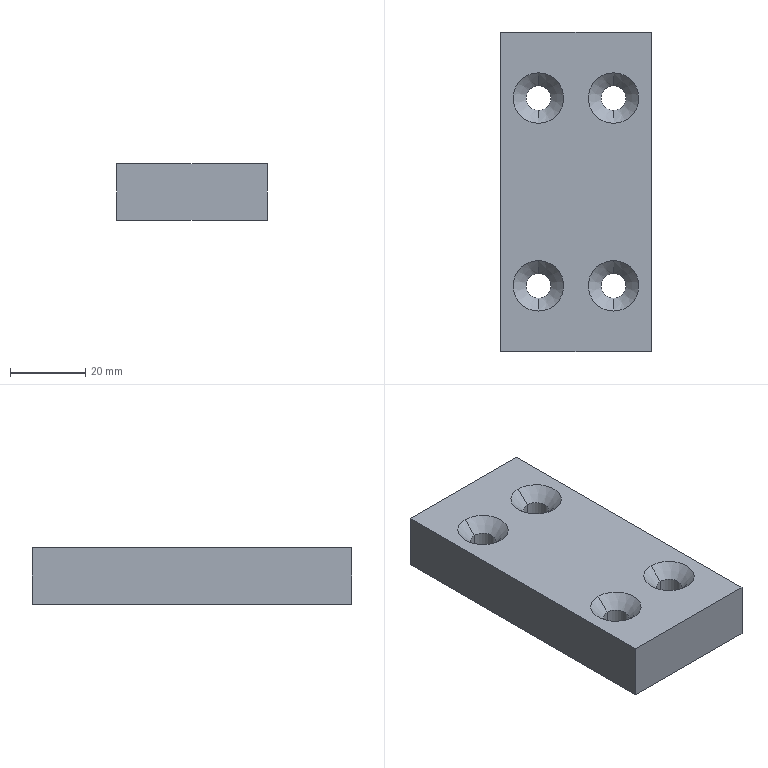Part | STEP file | 02-Rubber pad | 1 solid | 22 faces | box 40 x 85 x 15 mm | volume 48295 mm3 | cone 8 | cylinder 8 | plane 6 | commonest cylinder face diameters 6.6 x8
STEP:
#1=CARTESIAN_POINT('',(0.,0.,0.));
#2=DIRECTION('',(0.,0.,1.));
#3=DIRECTION('',(1.,0.,0.));
#4=AXIS2_PLACEMENT_3D('',#1,#2,#3);
#5=CARTESIAN_POINT('',(10.,-20.8,11.58));
#6=VERTEX_POINT('',#5);
#7=CARTESIAN_POINT('',(10.,-24.22,15.));
#8=VERTEX_POINT('',#7);
#9=CARTESIAN_POINT('',(10.,-24.22,15.));
#10=DIRECTION('',(0.,-0.7071,0.7071));
#11=VECTOR('',#10,1.);
#12=LINE('',#9,#11);
#13=CARTESIAN_POINT('',(10.,-17.5,15.));
#14=DIRECTION('',(0.,0.,1.));
#15=DIRECTION('',(0.,-1.,0.));
#16=AXIS2_PLACEMENT_3D('',#13,#14,#15);
#17=CONICAL_SURFACE('',#16,6.72,0.7854);
#18=CARTESIAN_POINT('',(6.283,0.));
#19=DIRECTION('',(0.,1.));
#20=VECTOR('',#19,1.);
#21=LINE('',#18,#20);
#22=(GEOMETRIC_REPRESENTATION_CONTEXT(2)PARAMETRIC_REPRESENTATION_CONTEXT()REPRESENTATION_CONTEXT('',''));
#23=DEFINITIONAL_REPRESENTATION('',(#21),#22);
#24=PCURVE('',#17,#23);
#25=CARTESIAN_POINT('',(10.,-17.5,15.));
#26=DIRECTION('',(0.,0.,1.));
#27=DIRECTION('',(0.,-1.,0.));
#28=AXIS2_PLACEMENT_3D('',#25,#26,#27);
#29=CONICAL_SURFACE('',#28,6.72,0.7854);
#30=CARTESIAN_POINT('',(0.,0.));
#31=DIRECTION('',(0.,1.));
#32=VECTOR('',#31,1.);
#33=LINE('',#30,#32);
#34=(GEOMETRIC_REPRESENTATION_CONTEXT(2)PARAMETRIC_REPRESENTATION_CONTEXT()REPRESENTATION_CONTEXT('',''));
#35=DEFINITIONAL_REPRESENTATION('',(#33),#34);
#36=PCURVE('',#29,#35);
#37=SURFACE_CURVE('',#12,(#24,#36),.PCURVE_S1.);
#38=EDGE_CURVE('',#6,#8,#37,.T.);
#39=ORIENTED_EDGE('',*,*,#38,.T.);
#40=CARTESIAN_POINT('',(10.,-10.78,15.));
#41=VERTEX_POINT('',#40);
#42=CARTESIAN_POINT('',(10.,-17.5,15.));
#43=DIRECTION('',(0.,0.,1.));
#44=DIRECTION('',(0.,-1.,0.));
#45=AXIS2_PLACEMENT_3D('',#42,#43,#44);
#46=CIRCLE('',#45,6.72);
#47=CARTESIAN_POINT('',(0.,0.));
#48=DIRECTION('',(1.,0.));
#49=VECTOR('',#48,1.);
#50=LINE('',#47,#49);
#51=(GEOMETRIC_REPRESENTATION_CONTEXT(2)PARAMETRIC_REPRESENTATION_CONTEXT()REPRESENTATION_CONTEXT('',''));
#52=DEFINITIONAL_REPRESENTATION('',(#50),#51);
#53=PCURVE('',#17,#52);
#54=CARTESIAN_POINT('',(0.,0.,15.));
#55=DIRECTION('',(0.,0.,1.));
#56=DIRECTION('',(1.,0.,0.));
#57=AXIS2_PLACEMENT_3D('',#54,#55,#56);
#58=PLANE('',#57);
#59=CARTESIAN_POINT('',(10.,-17.5));
#60=DIRECTION('',(0.,-1.));
#61=AXIS2_PLACEMENT_2D('',#59,#60);
#62=CIRCLE('',#61,6.72);
#63=(GEOMETRIC_REPRESENTATION_CONTEXT(2)PARAMETRIC_REPRESENTATION_CONTEXT()REPRESENTATION_CONTEXT('',''));
#64=DEFINITIONAL_REPRESENTATION('',(#62),#63);
#65=PCURVE('',#58,#64);
#66=SURFACE_CURVE('',#46,(#53,#65),.PCURVE_S1.);
#67=EDGE_CURVE('',#41,#8,#66,.T.);
#68=ORIENTED_EDGE('',*,*,#67,.F.);
#69=CARTESIAN_POINT('',(10.,-14.2,11.58));
#70=VERTEX_POINT('',#69);
#71=CARTESIAN_POINT('',(10.,-10.78,15.));
#72=DIRECTION('',(0.,0.7071,0.7071));
#73=VECTOR('',#72,1.);
#74=LINE('',#71,#73);
#75=CARTESIAN_POINT('',(3.142,0.));
#76=DIRECTION('',(0.,1.));
#77=VECTOR('',#76,1.);
#78=LINE('',#75,#77);
#79=(GEOMETRIC_REPRESENTATION_CONTEXT(2)PARAMETRIC_REPRESENTATION_CONTEXT()REPRESENTATION_CONTEXT('',''));
#80=DEFINITIONAL_REPRESENTATION('',(#78),#79);
#81=PCURVE('',#17,#80);
#82=CARTESIAN_POINT('',(3.142,0.));
#83=DIRECTION('',(0.,1.));
#84=VECTOR('',#83,1.);
#85=LINE('',#82,#84);
#86=(GEOMETRIC_REPRESENTATION_CONTEXT(2)PARAMETRIC_REPRESENTATION_CONTEXT()REPRESENTATION_CONTEXT('',''));
#87=DEFINITIONAL_REPRESENTATION('',(#85),#86);
#88=PCURVE('',#29,#87);
#89=SURFACE_CURVE('',#74,(#81,#88),.PCURVE_S1.);
#90=EDGE_CURVE('',#70,#41,#89,.T.);
#91=ORIENTED_EDGE('',*,*,#90,.F.);
#92=CARTESIAN_POINT('',(10.,-17.5,11.58));
#93=DIRECTION('',(0.,0.,1.));
#94=DIRECTION('',(0.,-1.,0.));
#95=AXIS2_PLACEMENT_3D('',#92,#93,#94);
#96=CIRCLE('',#95,3.3);
#97=CARTESIAN_POINT('',(0.,-3.42));
#98=DIRECTION('',(1.,0.));
#99=VECTOR('',#98,1.);
#100=LINE('',#97,#99);
#101=(GEOMETRIC_REPRESENTATION_CONTEXT(2)PARAMETRIC_REPRESENTATION_CONTEXT()REPRESENTATION_CONTEXT('',''));
#102=DEFINITIONAL_REPRESENTATION('',(#100),#101);
#103=PCURVE('',#17,#102);
#104=CARTESIAN_POINT('',(10.,-17.5,15.));
#105=DIRECTION('',(0.,0.,1.));
#106=DIRECTION('',(0.,-1.,0.));
#107=AXIS2_PLACEMENT_3D('',#104,#105,#106);
#108=CYLINDRICAL_SURFACE('',#107,3.3);
#109=CARTESIAN_POINT('',(0.,-3.42));
#110=DIRECTION('',(1.,0.));
#111=VECTOR('',#110,1.);
#112=LINE('',#109,#111);
#113=(GEOMETRIC_REPRESENTATION_CONTEXT(2)PARAMETRIC_REPRESENTATION_CONTEXT()REPRESENTATION_CONTEXT('',''));
#114=DEFINITIONAL_REPRESENTATION('',(#112),#113);
#115=PCURVE('',#108,#114);
#116=SURFACE_CURVE('',#96,(#103,#115),.PCURVE_S1.);
#117=EDGE_CURVE('',#70,#6,#116,.T.);
#118=ORIENTED_EDGE('',*,*,#117,.T.);
#119=EDGE_LOOP('',(#39,#68,#91,#118));
#120=FACE_BOUND('',#119,.F.);
#121=ADVANCED_FACE('',(#120),#17,.F.);
#122=CARTESIAN_POINT('',(10.,-20.8,0.));
#123=VERTEX_POINT('',#122);
#124=CARTESIAN_POINT('',(10.,-20.8,15.));
#125=DIRECTION('',(0.,0.,1.));
#126=VECTOR('',#125,1.);
#127=LINE('',#124,#126);
#128=CARTESIAN_POINT('',(6.283,0.));
#129=DIRECTION('',(0.,1.));
#130=VECTOR('',#129,1.);
#131=LINE('',#128,#130);
#132=(GEOMETRIC_REPRESENTATION_CONTEXT(2)PARAMETRIC_REPRESENTATION_CONTEXT()REPRESENTATION_CONTEXT('',''));
#133=DEFINITIONAL_REPRESENTATION('',(#131),#132);
#134=PCURVE('',#108,#133);
#135=CARTESIAN_POINT('',(10.,-17.5,15.));
#136=DIRECTION('',(0.,0.,1.));
#137=DIRECTION('',(0.,-1.,0.));
#138=AXIS2_PLACEMENT_3D('',#135,#136,#137);
#139=CYLINDRICAL_SURFACE('',#138,3.3);
#140=CARTESIAN_POINT('',(0.,0.));
#141=DIRECTION('',(0.,1.));
#142=VECTOR('',#141,1.);
#143=LINE('',#140,#142);
#144=(GEOMETRIC_REPRESENTATION_CONTEXT(2)PARAMETRIC_REPRESENTATION_CONTEXT()REPRESENTATION_CONTEXT('',''));
#145=DEFINITIONAL_REPRESENTATION('',(#143),#144);
#146=PCURVE('',#139,#145);
#147=SURFACE_CURVE('',#127,(#134,#146),.PCURVE_S1.);
#148=EDGE_CURVE('',#123,#6,#147,.T.);
#149=ORIENTED_EDGE('',*,*,#148,.T.);
#150=ORIENTED_EDGE('',*,*,#117,.F.);
#151=CARTESIAN_POINT('',(10.,-14.2,0.));
#152=VERTEX_POINT('',#151);
#153=CARTESIAN_POINT('',(10.,-14.2,15.));
#154=DIRECTION('',(0.,0.,1.));
#155=VECTOR('',#154,1.);
#156=LINE('',#153,#155);
#157=CARTESIAN_POINT('',(3.142,0.));
#158=DIRECTION('',(0.,1.));
#159=VECTOR('',#158,1.);
#160=LINE('',#157,#159);
#161=(GEOMETRIC_REPRESENTATION_CONTEXT(2)PARAMETRIC_REPRESENTATION_CONTEXT()REPRESENTATION_CONTEXT('',''));
#162=DEFINITIONAL_REPRESENTATION('',(#160),#161);
#163=PCURVE('',#108,#162);
#164=CARTESIAN_POINT('',(3.142,0.));
#165=DIRECTION('',(0.,1.));
#166=VECTOR('',#165,1.);
#167=LINE('',#164,#166);
#168=(GEOMETRIC_REPRESENTATION_CONTEXT(2)PARAMETRIC_REPRESENTATION_CONTEXT()REPRESENTATION_CONTEXT('',''));
#169=DEFINITIONAL_REPRESENTATION('',(#167),#168);
#170=PCURVE('',#139,#169);
#171=SURFACE_CURVE('',#156,(#163,#170),.PCURVE_S1.);
#172=EDGE_CURVE('',#152,#70,#171,.T.);
#173=ORIENTED_EDGE('',*,*,#172,.F.);
#174=CARTESIAN_POINT('',(10.,-17.5,0.));
#175=DIRECTION('',(0.,0.,1.));
#176=DIRECTION('',(-1.,0.,0.));
#177=AXIS2_PLACEMENT_3D('',#174,#175,#176);
#178=CIRCLE('',#177,3.3);
#179=CARTESIAN_POINT('',(-1.571,-15.));
#180=DIRECTION('',(1.,0.));
#181=VECTOR('',#180,1.);
#182=LINE('',#179,#181);
#183=(GEOMETRIC_REPRESENTATION_CONTEXT(2)PARAMETRIC_REPRESENTATION_CONTEXT()REPRESENTATION_CONTEXT('',''));
#184=DEFINITIONAL_REPRESENTATION('',(#182),#183);
#185=PCURVE('',#108,#184);
#186=CARTESIAN_POINT('',(0.,0.,0.));
#187=DIRECTION('',(0.,0.,1.));
#188=DIRECTION('',(1.,0.,0.));
#189=AXIS2_PLACEMENT_3D('',#186,#187,#188);
#190=PLANE('',#189);
#191=CARTESIAN_POINT('',(10.,-17.5));
#192=DIRECTION('',(-1.,0.));
#193=AXIS2_PLACEMENT_2D('',#191,#192);
#194=CIRCLE('',#193,3.3);
#195=(GEOMETRIC_REPRESENTATION_CONTEXT(2)PARAMETRIC_REPRESENTATION_CONTEXT()REPRESENTATION_CONTEXT('',''));
#196=DEFINITIONAL_REPRESENTATION('',(#194),#195);
#197=PCURVE('',#190,#196);
#198=SURFACE_CURVE('',#178,(#185,#197),.PCURVE_S1.);
#199=EDGE_CURVE('',#152,#123,#198,.T.);
#200=ORIENTED_EDGE('',*,*,#199,.T.);
#201=EDGE_LOOP('',(#149,#150,#173,#200));
#202=FACE_BOUND('',#201,.F.);
#203=ADVANCED_FACE('',(#202),#108,.F.);
#204=CARTESIAN_POINT('',(10.,-70.8,11.58));
#205=VERTEX_POINT('',#204);
#206=CARTESIAN_POINT('',(10.,-74.22,15.));
#207=VERTEX_POINT('',#206);
#208=CARTESIAN_POINT('',(10.,-74.22,15.));
#209=DIRECTION('',(0.,-0.7071,0.7071));
#210=VECTOR('',#209,1.);
#211=LINE('',#208,#210);
#212=CARTESIAN_POINT('',(10.,-67.5,15.));
#213=DIRECTION('',(0.,0.,1.));
#214=DIRECTION('',(0.,-1.,0.));
#215=AXIS2_PLACEMENT_3D('',#212,#213,#214);
#216=CONICAL_SURFACE('',#215,6.72,0.7854);
#217=CARTESIAN_POINT('',(6.283,0.));
#218=DIRECTION('',(0.,1.));
#219=VECTOR('',#218,1.);
#220=LINE('',#217,#219);
#221=(GEOMETRIC_REPRESENTATION_CONTEXT(2)PARAMETRIC_REPRESENTATION_CONTEXT()REPRESENTATION_CONTEXT('',''));
#222=DEFINITIONAL_REPRESENTATION('',(#220),#221);
#223=PCURVE('',#216,#222);
#224=CARTESIAN_POINT('',(10.,-67.5,15.));
#225=DIRECTION('',(0.,0.,1.));
#226=DIRECTION('',(0.,-1.,0.));
#227=AXIS2_PLACEMENT_3D('',#224,#225,#226);
#228=CONICAL_SURFACE('',#227,6.72,0.7854);
#229=CARTESIAN_POINT('',(0.,0.));
#230=DIRECTION('',(0.,1.));
#231=VECTOR('',#230,1.);
#232=LINE('',#229,#231);
#233=(GEOMETRIC_REPRESENTATION_CONTEXT(2)PARAMETRIC_REPRESENTATION_CONTEXT()REPRESENTATION_CONTEXT('',''));
#234=DEFINITIONAL_REPRESENTATION('',(#232),#233);
#235=PCURVE('',#228,#234);
#236=SURFACE_CURVE('',#211,(#223,#235),.PCURVE_S1.);
#237=EDGE_CURVE('',#205,#207,#236,.T.);
#238=ORIENTED_EDGE('',*,*,#237,.T.);
#239=CARTESIAN_POINT('',(10.,-60.78,15.));
#240=VERTEX_POINT('',#239);
#241=CARTESIAN_POINT('',(10.,-67.5,15.));
#242=DIRECTION('',(0.,0.,1.));
#243=DIRECTION('',(0.,-1.,0.));
#244=AXIS2_PLACEMENT_3D('',#241,#242,#243);
#245=CIRCLE('',#244,6.72);
#246=CARTESIAN_POINT('',(0.,0.));
#247=DIRECTION('',(1.,0.));
#248=VECTOR('',#247,1.);
#249=LINE('',#246,#248);
#250=(GEOMETRIC_REPRESENTATION_CONTEXT(2)PARAMETRIC_REPRESENTATION_CONTEXT()REPRESENTATION_CONTEXT('',''));
#251=DEFINITIONAL_REPRESENTATION('',(#249),#250);
#252=PCURVE('',#216,#251);
#253=CARTESIAN_POINT('',(10.,-67.5));
#254=DIRECTION('',(0.,-1.));
#255=AXIS2_PLACEMENT_2D('',#253,#254);
#256=CIRCLE('',#255,6.72);
#257=(GEOMETRIC_REPRESENTATION_CONTEXT(2)PARAMETRIC_REPRESENTATION_CONTEXT()REPRESENTATION_CONTEXT('',''));
#258=DEFINITIONAL_REPRESENTATION('',(#256),#257);
#259=PCURVE('',#58,#258);
#260=SURFACE_CURVE('',#245,(#252,#259),.PCURVE_S1.);
#261=EDGE_CURVE('',#240,#207,#260,.T.);
#262=ORIENTED_EDGE('',*,*,#261,.F.);
#263=CARTESIAN_POINT('',(10.,-64.2,11.58));
#264=VERTEX_POINT('',#263);
#265=CARTESIAN_POINT('',(10.,-60.78,15.));
#266=DIRECTION('',(0.,0.7071,0.7071));
#267=VECTOR('',#266,1.);
#268=LINE('',#265,#267);
#269=CARTESIAN_POINT('',(3.142,0.));
#270=DIRECTION('',(0.,1.));
#271=VECTOR('',#270,1.);
#272=LINE('',#269,#271);
#273=(GEOMETRIC_REPRESENTATION_CONTEXT(2)PARAMETRIC_REPRESENTATION_CONTEXT()REPRESENTATION_CONTEXT('',''));
#274=DEFINITIONAL_REPRESENTATION('',(#272),#273);
#275=PCURVE('',#216,#274);
#276=CARTESIAN_POINT('',(3.142,0.));
#277=DIRECTION('',(0.,1.));
#278=VECTOR('',#277,1.);
#279=LINE('',#276,#278);
#280=(GEOMETRIC_REPRESENTATION_CONTEXT(2)PARAMETRIC_REPRESENTATION_CONTEXT()REPRESENTATION_CONTEXT('',''));
#281=DEFINITIONAL_REPRESENTATION('',(#279),#280);
#282=PCURVE('',#228,#281);
#283=SURFACE_CURVE('',#268,(#275,#282),.PCURVE_S1.);
#284=EDGE_CURVE('',#264,#240,#283,.T.);
#285=ORIENTED_EDGE('',*,*,#284,.F.);
#286=CARTESIAN_POINT('',(10.,-67.5,11.58));
#287=DIRECTION('',(0.,0.,1.));
#288=DIRECTION('',(0.,-1.,0.));
#289=AXIS2_PLACEMENT_3D('',#286,#287,#288);
#290=CIRCLE('',#289,3.3);
#291=CARTESIAN_POINT('',(0.,-3.42));
#292=DIRECTION('',(1.,0.));
#293=VECTOR('',#292,1.);
#294=LINE('',#291,#293);
#295=(GEOMETRIC_REPRESENTATION_CONTEXT(2)PARAMETRIC_REPRESENTATION_CONTEXT()REPRESENTATION_CONTEXT('',''));
#296=DEFINITIONAL_REPRESENTATION('',(#294),#295);
#297=PCURVE('',#216,#296);
#298=CARTESIAN_POINT('',(10.,-67.5,15.));
#299=DIRECTION('',(0.,0.,1.));
#300=DIRECTION('',(0.,-1.,0.));
#301=AXIS2_PLACEMENT_3D('',#298,#299,#300);
#302=CYLINDRICAL_SURFACE('',#301,3.3);
#303=CARTESIAN_POINT('',(0.,-3.42));
#304=DIRECTION('',(1.,0.));
#305=VECTOR('',#304,1.);
#306=LINE('',#303,#305);
#307=(GEOMETRIC_REPRESENTATION_CONTEXT(2)PARAMETRIC_REPRESENTATION_CONTEXT()REPRESENTATION_CONTEXT('',''));
#308=DEFINITIONAL_REPRESENTATION('',(#306),#307);
#309=PCURVE('',#302,#308);
#310=SURFACE_CURVE('',#290,(#297,#309),.PCURVE_S1.);
#311=EDGE_CURVE('',#264,#205,#310,.T.);
#312=ORIENTED_EDGE('',*,*,#311,.T.);
#313=EDGE_LOOP('',(#238,#262,#285,#312));
#314=FACE_BOUND('',#313,.F.);
#315=ADVANCED_FACE('',(#314),#216,.F.);
#316=CARTESIAN_POINT('',(10.,-70.8,0.));
#317=VERTEX_POINT('',#316);
#318=CARTESIAN_POINT('',(10.,-70.8,15.));
#319=DIRECTION('',(0.,0.,1.));
#320=VECTOR('',#319,1.);
#321=LINE('',#318,#320);
#322=CARTESIAN_POINT('',(6.283,0.));
#323=DIRECTION('',(0.,1.));
#324=VECTOR('',#323,1.);
#325=LINE('',#322,#324);
#326=(GEOMETRIC_REPRESENTATION_CONTEXT(2)PARAMETRIC_REPRESENTATION_CONTEXT()REPRESENTATION_CONTEXT('',''));
#327=DEFINITIONAL_REPRESENTATION('',(#325),#326);
#328=PCURVE('',#302,#327);
#329=CARTESIAN_POINT('',(10.,-67.5,15.));
#330=DIRECTION('',(0.,0.,1.));
#331=DIRECTION('',(0.,-1.,0.));
#332=AXIS2_PLACEMENT_3D('',#329,#330,#331);
#333=CYLINDRICAL_SURFACE('',#332,3.3);
#334=CARTESIAN_POINT('',(0.,0.));
#335=DIRECTION('',(0.,1.));
#336=VECTOR('',#335,1.);
#337=LINE('',#334,#336);
#338=(GEOMETRIC_REPRESENTATION_CONTEXT(2)PARAMETRIC_REPRESENTATION_CONTEXT()REPRESENTATION_CONTEXT('',''));
#339=DEFINITIONAL_REPRESENTATION('',(#337),#338);
#340=PCURVE('',#333,#339);
#341=SURFACE_CURVE('',#321,(#328,#340),.PCURVE_S1.);
#342=EDGE_CURVE('',#317,#205,#341,.T.);
#343=ORIENTED_EDGE('',*,*,#342,.T.);
#344=ORIENTED_EDGE('',*,*,#311,.F.);
#345=CARTESIAN_POINT('',(10.,-64.2,0.));
#346=VERTEX_POINT('',#345);
#347=CARTESIAN_POINT('',(10.,-64.2,15.));
#348=DIRECTION('',(0.,0.,1.));
#349=VECTOR('',#348,1.);
#350=LINE('',#347,#349);
#351=CARTESIAN_POINT('',(3.142,0.));
#352=DIRECTION('',(0.,1.));
#353=VECTOR('',#352,1.);
#354=LINE('',#351,#353);
#355=(GEOMETRIC_REPRESENTATION_CONTEXT(2)PARAMETRIC_REPRESENTATION_CONTEXT()REPRESENTATION_CONTEXT('',''));
#356=DEFINITIONAL_REPRESENTATION('',(#354),#355);
#357=PCURVE('',#302,#356);
#358=CARTESIAN_POINT('',(3.142,0.));
#359=DIRECTION('',(0.,1.));
#360=VECTOR('',#359,1.);
#361=LINE('',#358,#360);
#362=(GEOMETRIC_REPRESENTATION_CONTEXT(2)PARAMETRIC_REPRESENTATION_CONTEXT()REPRESENTATION_CONTEXT('',''));
#363=DEFINITIONAL_REPRESENTATION('',(#361),#362);
#364=PCURVE('',#333,#363);
#365=SURFACE_CURVE('',#350,(#357,#364),.PCURVE_S1.);
#366=EDGE_CURVE('',#346,#264,#365,.T.);
#367=ORIENTED_EDGE('',*,*,#366,.F.);
#368=CARTESIAN_POINT('',(10.,-67.5,0.));
#369=DIRECTION('',(0.,0.,1.));
#370=DIRECTION('',(-1.,0.,0.));
#371=AXIS2_PLACEMENT_3D('',#368,#369,#370);
#372=CIRCLE('',#371,3.3);
#373=CARTESIAN_POINT('',(-1.571,-15.));
#374=DIRECTION('',(1.,0.));
#375=VECTOR('',#374,1.);
#376=LINE('',#373,#375);
#377=(GEOMETRIC_REPRESENTATION_CONTEXT(2)PARAMETRIC_REPRESENTATION_CONTEXT()REPRESENTATION_CONTEXT('',''));
#378=DEFINITIONAL_REPRESENTATION('',(#376),#377);
#379=PCURVE('',#302,#378);
#380=CARTESIAN_POINT('',(10.,-67.5));
#381=DIRECTION('',(-1.,0.));
#382=AXIS2_PLACEMENT_2D('',#380,#381);
#383=CIRCLE('',#382,3.3);
#384=(GEOMETRIC_REPRESENTATION_CONTEXT(2)PARAMETRIC_REPRESENTATION_CONTEXT()REPRESENTATION_CONTEXT('',''));
#385=DEFINITIONAL_REPRESENTATION('',(#383),#384);
#386=PCURVE('',#190,#385);
#387=SURFACE_CURVE('',#372,(#379,#386),.PCURVE_S1.);
#388=EDGE_CURVE('',#346,#317,#387,.T.);
#389=ORIENTED_EDGE('',*,*,#388,.T.);
#390=EDGE_LOOP('',(#343,#344,#367,#389));
#391=FACE_BOUND('',#390,.F.);
#392=ADVANCED_FACE('',(#391),#302,.F.);
#393=CARTESIAN_POINT('',(30.,-20.8,11.58));
#394=VERTEX_POINT('',#393);
#395=CARTESIAN_POINT('',(30.,-24.22,15.));
#396=VERTEX_POINT('',#395);
#397=CARTESIAN_POINT('',(30.,-24.22,15.));
#398=DIRECTION('',(0.,-0.7071,0.7071));
#399=VECTOR('',#398,1.);
#400=LINE('',#397,#399);
#401=CARTESIAN_POINT('',(30.,-17.5,15.));
#402=DIRECTION('',(0.,0.,1.));
#403=DIRECTION('',(0.,-1.,0.));
#404=AXIS2_PLACEMENT_3D('',#401,#402,#403);
#405=CONICAL_SURFACE('',#404,6.72,0.7854);
#406=CARTESIAN_POINT('',(6.283,0.));
#407=DIRECTION('',(0.,1.));
#408=VECTOR('',#407,1.);
#409=LINE('',#406,#408);
#410=(GEOMETRIC_REPRESENTATION_CONTEXT(2)PARAMETRIC_REPRESENTATION_CONTEXT()REPRESENTATION_CONTEXT('',''));
#411=DEFINITIONAL_REPRESENTATION('',(#409),#410);
#412=PCURVE('',#405,#411);
#413=CARTESIAN_POINT('',(30.,-17.5,15.));
#414=DIRECTION('',(0.,0.,1.));
#415=DIRECTION('',(0.,-1.,0.));
#416=AXIS2_PLACEMENT_3D('',#413,#414,#415);
#417=CONICAL_SURFACE('',#416,6.72,0.7854);
#418=CARTESIAN_POINT('',(0.,0.));
#419=DIRECTION('',(0.,1.));
#420=VECTOR('',#419,1.);
#421=LINE('',#418,#420);
#422=(GEOMETRIC_REPRESENTATION_CONTEXT(2)PARAMETRIC_REPRESENTATION_CONTEXT()REPRESENTATION_CONTEXT('',''));
#423=DEFINITIONAL_REPRESENTATION('',(#421),#422);
#424=PCURVE('',#417,#423);
#425=SURFACE_CURVE('',#400,(#412,#424),.PCURVE_S1.);
#426=EDGE_CURVE('',#394,#396,#425,.T.);
#427=ORIENTED_EDGE('',*,*,#426,.T.);
#428=CARTESIAN_POINT('',(30.,-10.78,15.));
#429=VERTEX_POINT('',#428);
#430=CARTESIAN_POINT('',(30.,-17.5,15.));
#431=DIRECTION('',(0.,0.,1.));
#432=DIRECTION('',(0.,-1.,0.));
#433=AXIS2_PLACEMENT_3D('',#430,#431,#432);
#434=CIRCLE('',#433,6.72);
#435=CARTESIAN_POINT('',(0.,0.));
#436=DIRECTION('',(1.,0.));
#437=VECTOR('',#436,1.);
#438=LINE('',#435,#437);
#439=(GEOMETRIC_REPRESENTATION_CONTEXT(2)PARAMETRIC_REPRESENTATION_CONTEXT()REPRESENTATION_CONTEXT('',''));
#440=DEFINITIONAL_REPRESENTATION('',(#438),#439);
#441=PCURVE('',#405,#440);
#442=CARTESIAN_POINT('',(30.,-17.5));
#443=DIRECTION('',(0.,-1.));
#444=AXIS2_PLACEMENT_2D('',#442,#443);
#445=CIRCLE('',#444,6.72);
#446=(GEOMETRIC_REPRESENTATION_CONTEXT(2)PARAMETRIC_REPRESENTATION_CONTEXT()REPRESENTATION_CONTEXT('',''));
#447=DEFINITIONAL_REPRESENTATION('',(#445),#446);
#448=PCURVE('',#58,#447);
#449=SURFACE_CURVE('',#434,(#441,#448),.PCURVE_S1.);
#450=EDGE_CURVE('',#429,#396,#449,.T.);
#451=ORIENTED_EDGE('',*,*,#450,.F.);
#452=CARTESIAN_POINT('',(30.,-14.2,11.58));
#453=VERTEX_POINT('',#452);
#454=CARTESIAN_POINT('',(30.,-10.78,15.));
#455=DIRECTION('',(0.,0.7071,0.7071));
#456=VECTOR('',#455,1.);
#457=LINE('',#454,#456);
#458=CARTESIAN_POINT('',(3.142,0.));
#459=DIRECTION('',(0.,1.));
#460=VECTOR('',#459,1.);
#461=LINE('',#458,#460);
#462=(GEOMETRIC_REPRESENTATION_CONTEXT(2)PARAMETRIC_REPRESENTATION_CONTEXT()REPRESENTATION_CONTEXT('',''));
#463=DEFINITIONAL_REPRESENTATION('',(#461),#462);
#464=PCURVE('',#405,#463);
#465=CARTESIAN_POINT('',(3.142,0.));
#466=DIRECTION('',(0.,1.));
#467=VECTOR('',#466,1.);
#468=LINE('',#465,#467);
#469=(GEOMETRIC_REPRESENTATION_CONTEXT(2)PARAMETRIC_REPRESENTATION_CONTEXT()REPRESENTATION_CONTEXT('',''));
#470=DEFINITIONAL_REPRESENTATION('',(#468),#469);
#471=PCURVE('',#417,#470);
#472=SURFACE_CURVE('',#457,(#464,#471),.PCURVE_S1.);
#473=EDGE_CURVE('',#453,#429,#472,.T.);
#474=ORIENTED_EDGE('',*,*,#473,.F.);
#475=CARTESIAN_POINT('',(30.,-17.5,11.58));
#476=DIRECTION('',(0.,0.,1.));
#477=DIRECTION('',(0.,-1.,0.));
#478=AXIS2_PLACEMENT_3D('',#475,#476,#477);
#479=CIRCLE('',#478,3.3);
#480=CARTESIAN_POINT('',(0.,-3.42));
#481=DIRECTION('',(1.,0.));
#482=VECTOR('',#481,1.);
#483=LINE('',#480,#482);
#484=(GEOMETRIC_REPRESENTATION_CONTEXT(2)PARAMETRIC_REPRESENTATION_CONTEXT()REPRESENTATION_CONTEXT('',''));
#485=DEFINITIONAL_REPRESENTATION('',(#483),#484);
#486=PCURVE('',#405,#485);
#487=CARTESIAN_POINT('',(30.,-17.5,15.));
#488=DIRECTION('',(0.,0.,1.));
#489=DIRECTION('',(0.,-1.,0.));
#490=AXIS2_PLACEMENT_3D('',#487,#488,#489);
#491=CYLINDRICAL_SURFACE('',#490,3.3);
#492=CARTESIAN_POINT('',(0.,-3.42));
#493=DIRECTION('',(1.,0.));
#494=VECTOR('',#493,1.);
#495=LINE('',#492,#494);
#496=(GEOMETRIC_REPRESENTATION_CONTEXT(2)PARAMETRIC_REPRESENTATION_CONTEXT()REPRESENTATION_CONTEXT('',''));
#497=DEFINITIONAL_REPRESENTATION('',(#495),#496);
#498=PCURVE('',#491,#497);
#499=SURFACE_CURVE('',#479,(#486,#498),.PCURVE_S1.);
#500=EDGE_CURVE('',#453,#394,#499,.T.);
#501=ORIENTED_EDGE('',*,*,#500,.T.);
#502=EDGE_LOOP('',(#427,#451,#474,#501));
#503=FACE_BOUND('',#502,.F.);
#504=ADVANCED_FACE('',(#503),#405,.F.);
#505=CARTESIAN_POINT('',(30.,-20.8,0.));
#506=VERTEX_POINT('',#505);
#507=CARTESIAN_POINT('',(30.,-20.8,15.));
#508=DIRECTION('',(0.,0.,1.));
#509=VECTOR('',#508,1.);
#510=LINE('',#507,#509);
#511=CARTESIAN_POINT('',(6.283,0.));
#512=DIRECTION('',(0.,1.));
#513=VECTOR('',#512,1.);
#514=LINE('',#511,#513);
#515=(GEOMETRIC_REPRESENTATION_CONTEXT(2)PARAMETRIC_REPRESENTATION_CONTEXT()REPRESENTATION_CONTEXT('',''));
#516=DEFINITIONAL_REPRESENTATION('',(#514),#515);
#517=PCURVE('',#491,#516);
#518=CARTESIAN_POINT('',(30.,-17.5,15.));
#519=DIRECTION('',(0.,0.,1.));
#520=DIRECTION('',(0.,-1.,0.));
#521=AXIS2_PLACEMENT_3D('',#518,#519,#520);
#522=CYLINDRICAL_SURFACE('',#521,3.3);
#523=CARTESIAN_POINT('',(0.,0.));
#524=DIRECTION('',(0.,1.));
#525=VECTOR('',#524,1.);
#526=LINE('',#523,#525);
#527=(GEOMETRIC_REPRESENTATION_CONTEXT(2)PARAMETRIC_REPRESENTATION_CONTEXT()REPRESENTATION_CONTEXT('',''));
#528=DEFINITIONAL_REPRESENTATION('',(#526),#527);
#529=PCURVE('',#522,#528);
#530=SURFACE_CURVE('',#510,(#517,#529),.PCURVE_S1.);
#531=EDGE_CURVE('',#506,#394,#530,.T.);
#532=ORIENTED_EDGE('',*,*,#531,.T.);
#533=ORIENTED_EDGE('',*,*,#500,.F.);
#534=CARTESIAN_POINT('',(30.,-14.2,0.));
#535=VERTEX_POINT('',#534);
#536=CARTESIAN_POINT('',(30.,-14.2,15.));
#537=DIRECTION('',(0.,0.,1.));
#538=VECTOR('',#537,1.);
#539=LINE('',#536,#538);
#540=CARTESIAN_POINT('',(3.142,0.));
#541=DIRECTION('',(0.,1.));
#542=VECTOR('',#541,1.);
#543=LINE('',#540,#542);
#544=(GEOMETRIC_REPRESENTATION_CONTEXT(2)PARAMETRIC_REPRESENTATION_CONTEXT()REPRESENTATION_CONTEXT('',''));
#545=DEFINITIONAL_REPRESENTATION('',(#543),#544);
#546=PCURVE('',#491,#545);
#547=CARTESIAN_POINT('',(3.142,0.));
#548=DIRECTION('',(0.,1.));
#549=VECTOR('',#548,1.);
#550=LINE('',#547,#549);
#551=(GEOMETRIC_REPRESENTATION_CONTEXT(2)PARAMETRIC_REPRESENTATION_CONTEXT()REPRESENTATION_CONTEXT('',''));
#552=DEFINITIONAL_REPRESENTATION('',(#550),#551);
#553=PCURVE('',#522,#552);
#554=SURFACE_CURVE('',#539,(#546,#553),.PCURVE_S1.);
#555=EDGE_CURVE('',#535,#453,#554,.T.);
#556=ORIENTED_EDGE('',*,*,#555,.F.);
#557=CARTESIAN_POINT('',(30.,-17.5,0.));
#558=DIRECTION('',(0.,0.,1.));
#559=DIRECTION('',(-1.,0.,0.));
#560=AXIS2_PLACEMENT_3D('',#557,#558,#559);
#561=CIRCLE('',#560,3.3);
#562=CARTESIAN_POINT('',(-1.571,-15.));
#563=DIRECTION('',(1.,0.));
#564=VECTOR('',#563,1.);
#565=LINE('',#562,#564);
#566=(GEOMETRIC_REPRESENTATION_CONTEXT(2)PARAMETRIC_REPRESENTATION_CONTEXT()REPRESENTATION_CONTEXT('',''));
#567=DEFINITIONAL_REPRESENTATION('',(#565),#566);
#568=PCURVE('',#491,#567);
#569=CARTESIAN_POINT('',(30.,-17.5));
#570=DIRECTION('',(-1.,0.));
#571=AXIS2_PLACEMENT_2D('',#569,#570);
#572=CIRCLE('',#571,3.3);
#573=(GEOMETRIC_REPRESENTATION_CONTEXT(2)PARAMETRIC_REPRESENTATION_CONTEXT()REPRESENTATION_CONTEXT('',''));
#574=DEFINITIONAL_REPRESENTATION('',(#572),#573);
#575=PCURVE('',#190,#574);
#576=SURFACE_CURVE('',#561,(#568,#575),.PCURVE_S1.);
#577=EDGE_CURVE('',#535,#506,#576,.T.);
#578=ORIENTED_EDGE('',*,*,#577,.T.);
#579=EDGE_LOOP('',(#532,#533,#556,#578));
#580=FACE_BOUND('',#579,.F.);
#581=ADVANCED_FACE('',(#580),#491,.F.);
#582=CARTESIAN_POINT('',(30.,-70.8,11.58));
#583=VERTEX_POINT('',#582);
#584=CARTESIAN_POINT('',(30.,-74.22,15.));
#585=VERTEX_POINT('',#584);
#586=CARTESIAN_POINT('',(30.,-74.22,15.));
#587=DIRECTION('',(0.,-0.7071,0.7071));
#588=VECTOR('',#587,1.);
#589=LINE('',#586,#588);
#590=CARTESIAN_POINT('',(30.,-67.5,15.));
#591=DIRECTION('',(0.,0.,1.));
#592=DIRECTION('',(0.,-1.,0.));
#593=AXIS2_PLACEMENT_3D('',#590,#591,#592);
#594=CONICAL_SURFACE('',#593,6.72,0.7854);
#595=CARTESIAN_POINT('',(6.283,0.));
#596=DIRECTION('',(0.,1.));
#597=VECTOR('',#596,1.);
#598=LINE('',#595,#597);
#599=(GEOMETRIC_REPRESENTATION_CONTEXT(2)PARAMETRIC_REPRESENTATION_CONTEXT()REPRESENTATION_CONTEXT('',''));
#600=DEFINITIONAL_REPRESENTATION('',(#598),#599);
#601=PCURVE('',#594,#600);
#602=CARTESIAN_POINT('',(30.,-67.5,15.));
#603=DIRECTION('',(0.,0.,1.));
#604=DIRECTION('',(0.,-1.,0.));
#605=AXIS2_PLACEMENT_3D('',#602,#603,#604);
#606=CONICAL_SURFACE('',#605,6.72,0.7854);
#607=CARTESIAN_POINT('',(0.,0.));
#608=DIRECTION('',(0.,1.));
#609=VECTOR('',#608,1.);
#610=LINE('',#607,#609);
#611=(GEOMETRIC_REPRESENTATION_CONTEXT(2)PARAMETRIC_REPRESENTATION_CONTEXT()REPRESENTATION_CONTEXT('',''));
#612=DEFINITIONAL_REPRESENTATION('',(#610),#611);
#613=PCURVE('',#606,#612);
#614=SURFACE_CURVE('',#589,(#601,#613),.PCURVE_S1.);
#615=EDGE_CURVE('',#583,#585,#614,.T.);
#616=ORIENTED_EDGE('',*,*,#615,.T.);
#617=CARTESIAN_POINT('',(30.,-60.78,15.));
#618=VERTEX_POINT('',#617);
#619=CARTESIAN_POINT('',(30.,-67.5,15.));
#620=DIRECTION('',(0.,0.,1.));
#621=DIRECTION('',(0.,-1.,0.));
#622=AXIS2_PLACEMENT_3D('',#619,#620,#621);
#623=CIRCLE('',#622,6.72);
#624=CARTESIAN_POINT('',(0.,0.));
#625=DIRECTION('',(1.,0.));
#626=VECTOR('',#625,1.);
#627=LINE('',#624,#626);
#628=(GEOMETRIC_REPRESENTATION_CONTEXT(2)PARAMETRIC_REPRESENTATION_CONTEXT()REPRESENTATION_CONTEXT('',''));
#629=DEFINITIONAL_REPRESENTATION('',(#627),#628);
#630=PCURVE('',#594,#629);
#631=CARTESIAN_POINT('',(30.,-67.5));
#632=DIRECTION('',(0.,-1.));
#633=AXIS2_PLACEMENT_2D('',#631,#632);
#634=CIRCLE('',#633,6.72);
#635=(GEOMETRIC_REPRESENTATION_CONTEXT(2)PARAMETRIC_REPRESENTATION_CONTEXT()REPRESENTATION_CONTEXT('',''));
#636=DEFINITIONAL_REPRESENTATION('',(#634),#635);
#637=PCURVE('',#58,#636);
#638=SURFACE_CURVE('',#623,(#630,#637),.PCURVE_S1.);
#639=EDGE_CURVE('',#618,#585,#638,.T.);
#640=ORIENTED_EDGE('',*,*,#639,.F.);
#641=CARTESIAN_POINT('',(30.,-64.2,11.58));
#642=VERTEX_POINT('',#641);
#643=CARTESIAN_POINT('',(30.,-60.78,15.));
#644=DIRECTION('',(0.,0.7071,0.7071));
#645=VECTOR('',#644,1.);
#646=LINE('',#643,#645);
#647=CARTESIAN_POINT('',(3.142,0.));
#648=DIRECTION('',(0.,1.));
#649=VECTOR('',#648,1.);
#650=LINE('',#647,#649);
#651=(GEOMETRIC_REPRESENTATION_CONTEXT(2)PARAMETRIC_REPRESENTATION_CONTEXT()REPRESENTATION_CONTEXT('',''));
#652=DEFINITIONAL_REPRESENTATION('',(#650),#651);
#653=PCURVE('',#594,#652);
#654=CARTESIAN_POINT('',(3.142,0.));
#655=DIRECTION('',(0.,1.));
#656=VECTOR('',#655,1.);
#657=LINE('',#654,#656);
#658=(GEOMETRIC_REPRESENTATION_CONTEXT(2)PARAMETRIC_REPRESENTATION_CONTEXT()REPRESENTATION_CONTEXT('',''));
#659=DEFINITIONAL_REPRESENTATION('',(#657),#658);
#660=PCURVE('',#606,#659);
#661=SURFACE_CURVE('',#646,(#653,#660),.PCURVE_S1.);
#662=EDGE_CURVE('',#642,#618,#661,.T.);
#663=ORIENTED_EDGE('',*,*,#662,.F.);
#664=CARTESIAN_POINT('',(30.,-67.5,11.58));
#665=DIRECTION('',(0.,0.,1.));
#666=DIRECTION('',(0.,-1.,0.));
#667=AXIS2_PLACEMENT_3D('',#664,#665,#666);
#668=CIRCLE('',#667,3.3);
#669=CARTESIAN_POINT('',(0.,-3.42));
#670=DIRECTION('',(1.,0.));
#671=VECTOR('',#670,1.);
#672=LINE('',#669,#671);
#673=(GEOMETRIC_REPRESENTATION_CONTEXT(2)PARAMETRIC_REPRESENTATION_CONTEXT()REPRESENTATION_CONTEXT('',''));
#674=DEFINITIONAL_REPRESENTATION('',(#672),#673);
#675=PCURVE('',#594,#674);
#676=CARTESIAN_POINT('',(30.,-67.5,15.));
#677=DIRECTION('',(0.,0.,1.));
#678=DIRECTION('',(0.,-1.,0.));
#679=AXIS2_PLACEMENT_3D('',#676,#677,#678);
#680=CYLINDRICAL_SURFACE('',#679,3.3);
#681=CARTESIAN_POINT('',(0.,-3.42));
#682=DIRECTION('',(1.,0.));
#683=VECTOR('',#682,1.);
#684=LINE('',#681,#683);
#685=(GEOMETRIC_REPRESENTATION_CONTEXT(2)PARAMETRIC_REPRESENTATION_CONTEXT()REPRESENTATION_CONTEXT('',''));
#686=DEFINITIONAL_REPRESENTATION('',(#684),#685);
#687=PCURVE('',#680,#686);
#688=SURFACE_CURVE('',#668,(#675,#687),.PCURVE_S1.);
#689=EDGE_CURVE('',#642,#583,#688,.T.);
#690=ORIENTED_EDGE('',*,*,#689,.T.);
#691=EDGE_LOOP('',(#616,#640,#663,#690));
#692=FACE_BOUND('',#691,.F.);
#693=ADVANCED_FACE('',(#692),#594,.F.);
#694=CARTESIAN_POINT('',(30.,-70.8,0.));
#695=VERTEX_POINT('',#694);
#696=CARTESIAN_POINT('',(30.,-70.8,15.));
#697=DIRECTION('',(0.,0.,1.));
#698=VECTOR('',#697,1.);
#699=LINE('',#696,#698);
#700=CARTESIAN_POINT('',(6.283,0.));
#701=DIRECTION('',(0.,1.));
#702=VECTOR('',#701,1.);
#703=LINE('',#700,#702);
#704=(GEOMETRIC_REPRESENTATION_CONTEXT(2)PARAMETRIC_REPRESENTATION_CONTEXT()REPRESENTATION_CONTEXT('',''));
#705=DEFINITIONAL_REPRESENTATION('',(#703),#704);
#706=PCURVE('',#680,#705);
#707=CARTESIAN_POINT('',(30.,-67.5,15.));
#708=DIRECTION('',(0.,0.,1.));
#709=DIRECTION('',(0.,-1.,0.));
#710=AXIS2_PLACEMENT_3D('',#707,#708,#709);
#711=CYLINDRICAL_SURFACE('',#710,3.3);
#712=CARTESIAN_POINT('',(0.,0.));
#713=DIRECTION('',(0.,1.));
#714=VECTOR('',#713,1.);
#715=LINE('',#712,#714);
#716=(GEOMETRIC_REPRESENTATION_CONTEXT(2)PARAMETRIC_REPRESENTATION_CONTEXT()REPRESENTATION_CONTEXT('',''));
#717=DEFINITIONAL_REPRESENTATION('',(#715),#716);
#718=PCURVE('',#711,#717);
#719=SURFACE_CURVE('',#699,(#706,#718),.PCURVE_S1.);
#720=EDGE_CURVE('',#695,#583,#719,.T.);
#721=ORIENTED_EDGE('',*,*,#720,.T.);
#722=ORIENTED_EDGE('',*,*,#689,.F.);
#723=CARTESIAN_POINT('',(30.,-64.2,0.));
#724=VERTEX_POINT('',#723);
#725=CARTESIAN_POINT('',(30.,-64.2,15.));
#726=DIRECTION('',(0.,0.,1.));
#727=VECTOR('',#726,1.);
#728=LINE('',#725,#727);
#729=CARTESIAN_POINT('',(3.142,0.));
#730=DIRECTION('',(0.,1.));
#731=VECTOR('',#730,1.);
#732=LINE('',#729,#731);
#733=(GEOMETRIC_REPRESENTATION_CONTEXT(2)PARAMETRIC_REPRESENTATION_CONTEXT()REPRESENTATION_CONTEXT('',''));
#734=DEFINITIONAL_REPRESENTATION('',(#732),#733);
#735=PCURVE('',#680,#734);
#736=CARTESIAN_POINT('',(3.142,0.));
#737=DIRECTION('',(0.,1.));
#738=VECTOR('',#737,1.);
#739=LINE('',#736,#738);
#740=(GEOMETRIC_REPRESENTATION_CONTEXT(2)PARAMETRIC_REPRESENTATION_CONTEXT()REPRESENTATION_CONTEXT('',''));
#741=DEFINITIONAL_REPRESENTATION('',(#739),#740);
#742=PCURVE('',#711,#741);
#743=SURFACE_CURVE('',#728,(#735,#742),.PCURVE_S1.);
#744=EDGE_CURVE('',#724,#642,#743,.T.);
#745=ORIENTED_EDGE('',*,*,#744,.F.);
#746=CARTESIAN_POINT('',(30.,-67.5,0.));
#747=DIRECTION('',(0.,0.,1.));
#748=DIRECTION('',(-1.,0.,0.));
#749=AXIS2_PLACEMENT_3D('',#746,#747,#748);
#750=CIRCLE('',#749,3.3);
#751=CARTESIAN_POINT('',(-1.571,-15.));
#752=DIRECTION('',(1.,0.));
#753=VECTOR('',#752,1.);
#754=LINE('',#751,#753);
#755=(GEOMETRIC_REPRESENTATION_CONTEXT(2)PARAMETRIC_REPRESENTATION_CONTEXT()REPRESENTATION_CONTEXT('',''));
#756=DEFINITIONAL_REPRESENTATION('',(#754),#755);
#757=PCURVE('',#680,#756);
#758=CARTESIAN_POINT('',(30.,-67.5));
#759=DIRECTION('',(-1.,0.));
#760=AXIS2_PLACEMENT_2D('',#758,#759);
#761=CIRCLE('',#760,3.3);
#762=(GEOMETRIC_REPRESENTATION_CONTEXT(2)PARAMETRIC_REPRESENTATION_CONTEXT()REPRESENTATION_CONTEXT('',''));
#763=DEFINITIONAL_REPRESENTATION('',(#761),#762);
#764=PCURVE('',#190,#763);
#765=SURFACE_CURVE('',#750,(#757,#764),.PCURVE_S1.);
#766=EDGE_CURVE('',#724,#695,#765,.T.);
#767=ORIENTED_EDGE('',*,*,#766,.T.);
#768=EDGE_LOOP('',(#721,#722,#745,#767));
#769=FACE_BOUND('',#768,.F.);
#770=ADVANCED_FACE('',(#769),#680,.F.);
#771=CARTESIAN_POINT('',(0.,0.,0.));
#772=VERTEX_POINT('',#771);
#773=CARTESIAN_POINT('',(0.,-85.,0.));
#774=VERTEX_POINT('',#773);
#775=CARTESIAN_POINT('',(0.,0.,0.));
#776=DIRECTION('',(0.,-1.,0.));
#777=VECTOR('',#776,1.);
#778=LINE('',#775,#777);
#779=CARTESIAN_POINT('',(0.,0.,15.));
#780=DIRECTION('',(1.,0.,0.));
#781=DIRECTION('',(0.,1.,0.));
#782=AXIS2_PLACEMENT_3D('',#779,#780,#781);
#783=PLANE('',#782);
#784=CARTESIAN_POINT('',(0.,-15.));
#785=DIRECTION('',(-1.,0.));
#786=VECTOR('',#785,1.);
#787=LINE('',#784,#786);
#788=(GEOMETRIC_REPRESENTATION_CONTEXT(2)PARAMETRIC_REPRESENTATION_CONTEXT()REPRESENTATION_CONTEXT('',''));
#789=DEFINITIONAL_REPRESENTATION('',(#787),#788);
#790=PCURVE('',#783,#789);
#791=CARTESIAN_POINT('',(0.,0.));
#792=DIRECTION('',(0.,-1.));
#793=VECTOR('',#792,1.);
#794=LINE('',#791,#793);
#795=(GEOMETRIC_REPRESENTATION_CONTEXT(2)PARAMETRIC_REPRESENTATION_CONTEXT()REPRESENTATION_CONTEXT('',''));
#796=DEFINITIONAL_REPRESENTATION('',(#794),#795);
#797=PCURVE('',#190,#796);
#798=SURFACE_CURVE('',#778,(#790,#797),.PCURVE_S1.);
#799=EDGE_CURVE('',#772,#774,#798,.T.);
#800=ORIENTED_EDGE('',*,*,#799,.T.);
#801=CARTESIAN_POINT('',(0.,-85.,15.));
#802=VERTEX_POINT('',#801);
#803=CARTESIAN_POINT('',(0.,-85.,15.));
#804=DIRECTION('',(0.,0.,-1.));
#805=VECTOR('',#804,1.);
#806=LINE('',#803,#805);
#807=CARTESIAN_POINT('',(-85.,0.));
#808=DIRECTION('',(0.,-1.));
#809=VECTOR('',#808,1.);
#810=LINE('',#807,#809);
#811=(GEOMETRIC_REPRESENTATION_CONTEXT(2)PARAMETRIC_REPRESENTATION_CONTEXT()REPRESENTATION_CONTEXT('',''));
#812=DEFINITIONAL_REPRESENTATION('',(#810),#811);
#813=PCURVE('',#783,#812);
#814=CARTESIAN_POINT('',(0.,-85.,15.));
#815=DIRECTION('',(0.,1.,0.));
#816=DIRECTION('',(0.,0.,1.));
#817=AXIS2_PLACEMENT_3D('',#814,#815,#816);
#818=PLANE('',#817);
#819=CARTESIAN_POINT('',(0.,0.));
#820=DIRECTION('',(-1.,0.));
#821=VECTOR('',#820,1.);
#822=LINE('',#819,#821);
#823=(GEOMETRIC_REPRESENTATION_CONTEXT(2)PARAMETRIC_REPRESENTATION_CONTEXT()REPRESENTATION_CONTEXT('',''));
#824=DEFINITIONAL_REPRESENTATION('',(#822),#823);
#825=PCURVE('',#818,#824);
#826=SURFACE_CURVE('',#806,(#813,#825),.PCURVE_S1.);
#827=EDGE_CURVE('',#802,#774,#826,.T.);
#828=ORIENTED_EDGE('',*,*,#827,.F.);
#829=CARTESIAN_POINT('',(0.,0.,15.));
#830=VERTEX_POINT('',#829);
#831=CARTESIAN_POINT('',(0.,0.,15.));
#832=DIRECTION('',(0.,-1.,0.));
#833=VECTOR('',#832,1.);
#834=LINE('',#831,#833);
#835=CARTESIAN_POINT('',(0.,0.));
#836=DIRECTION('',(-1.,0.));
#837=VECTOR('',#836,1.);
#838=LINE('',#835,#837);
#839=(GEOMETRIC_REPRESENTATION_CONTEXT(2)PARAMETRIC_REPRESENTATION_CONTEXT()REPRESENTATION_CONTEXT('',''));
#840=DEFINITIONAL_REPRESENTATION('',(#838),#839);
#841=PCURVE('',#783,#840);
#842=CARTESIAN_POINT('',(0.,0.));
#843=DIRECTION('',(0.,-1.));
#844=VECTOR('',#843,1.);
#845=LINE('',#842,#844);
#846=(GEOMETRIC_REPRESENTATION_CONTEXT(2)PARAMETRIC_REPRESENTATION_CONTEXT()REPRESENTATION_CONTEXT('',''));
#847=DEFINITIONAL_REPRESENTATION('',(#845),#846);
#848=PCURVE('',#58,#847);
#849=SURFACE_CURVE('',#834,(#841,#848),.PCURVE_S1.);
#850=EDGE_CURVE('',#830,#802,#849,.T.);
#851=ORIENTED_EDGE('',*,*,#850,.F.);
#852=CARTESIAN_POINT('',(0.,0.,15.));
#853=DIRECTION('',(0.,0.,-1.));
#854=VECTOR('',#853,1.);
#855=LINE('',#852,#854);
#856=CARTESIAN_POINT('',(0.,0.));
#857=DIRECTION('',(0.,-1.));
#858=VECTOR('',#857,1.);
#859=LINE('',#856,#858);
#860=(GEOMETRIC_REPRESENTATION_CONTEXT(2)PARAMETRIC_REPRESENTATION_CONTEXT()REPRESENTATION_CONTEXT('',''));
#861=DEFINITIONAL_REPRESENTATION('',(#859),#860);
#862=PCURVE('',#783,#861);
#863=CARTESIAN_POINT('',(0.,0.,15.));
#864=DIRECTION('',(0.,-1.,0.));
#865=DIRECTION('',(0.,0.,-1.));
#866=AXIS2_PLACEMENT_3D('',#863,#864,#865);
#867=PLANE('',#866);
#868=CARTESIAN_POINT('',(0.,0.));
#869=DIRECTION('',(1.,0.));
#870=VECTOR('',#869,1.);
#871=LINE('',#868,#870);
#872=(GEOMETRIC_REPRESENTATION_CONTEXT(2)PARAMETRIC_REPRESENTATION_CONTEXT()REPRESENTATION_CONTEXT('',''));
#873=DEFINITIONAL_REPRESENTATION('',(#871),#872);
#874=PCURVE('',#867,#873);
#875=SURFACE_CURVE('',#855,(#862,#874),.PCURVE_S1.);
#876=EDGE_CURVE('',#830,#772,#875,.T.);
#877=ORIENTED_EDGE('',*,*,#876,.T.);
#878=EDGE_LOOP('',(#800,#828,#851,#877));
#879=FACE_BOUND('',#878,.T.);
#880=ADVANCED_FACE('',(#879),#783,.F.);
#881=CARTESIAN_POINT('',(40.,-85.,0.));
#882=VERTEX_POINT('',#881);
#883=CARTESIAN_POINT('',(0.,-85.,0.));
#884=DIRECTION('',(1.,0.,0.));
#885=VECTOR('',#884,1.);
#886=LINE('',#883,#885);
#887=CARTESIAN_POINT('',(-15.,0.));
#888=DIRECTION('',(0.,1.));
#889=VECTOR('',#888,1.);
#890=LINE('',#887,#889);
#891=(GEOMETRIC_REPRESENTATION_CONTEXT(2)PARAMETRIC_REPRESENTATION_CONTEXT()REPRESENTATION_CONTEXT('',''));
#892=DEFINITIONAL_REPRESENTATION('',(#890),#891);
#893=PCURVE('',#818,#892);
#894=CARTESIAN_POINT('',(0.,-85.));
#895=DIRECTION('',(1.,0.));
#896=VECTOR('',#895,1.);
#897=LINE('',#894,#896);
#898=(GEOMETRIC_REPRESENTATION_CONTEXT(2)PARAMETRIC_REPRESENTATION_CONTEXT()REPRESENTATION_CONTEXT('',''));
#899=DEFINITIONAL_REPRESENTATION('',(#897),#898);
#900=PCURVE('',#190,#899);
#901=SURFACE_CURVE('',#886,(#893,#900),.PCURVE_S1.);
#902=EDGE_CURVE('',#774,#882,#901,.T.);
#903=ORIENTED_EDGE('',*,*,#902,.T.);
#904=CARTESIAN_POINT('',(40.,-85.,15.));
#905=VERTEX_POINT('',#904);
#906=CARTESIAN_POINT('',(40.,-85.,15.));
#907=DIRECTION('',(0.,0.,-1.));
#908=VECTOR('',#907,1.);
#909=LINE('',#906,#908);
#910=CARTESIAN_POINT('',(0.,40.));
#911=DIRECTION('',(-1.,0.));
#912=VECTOR('',#911,1.);
#913=LINE('',#910,#912);
#914=(GEOMETRIC_REPRESENTATION_CONTEXT(2)PARAMETRIC_REPRESENTATION_CONTEXT()REPRESENTATION_CONTEXT('',''));
#915=DEFINITIONAL_REPRESENTATION('',(#913),#914);
#916=PCURVE('',#818,#915);
#917=CARTESIAN_POINT('',(40.,0.,15.));
#918=DIRECTION('',(-1.,0.,0.));
#919=DIRECTION('',(0.,-1.,0.));
#920=AXIS2_PLACEMENT_3D('',#917,#918,#919);
#921=PLANE('',#920);
#922=CARTESIAN_POINT('',(85.,0.));
#923=DIRECTION('',(0.,-1.));
#924=VECTOR('',#923,1.);
#925=LINE('',#922,#924);
#926=(GEOMETRIC_REPRESENTATION_CONTEXT(2)PARAMETRIC_REPRESENTATION_CONTEXT()REPRESENTATION_CONTEXT('',''));
#927=DEFINITIONAL_REPRESENTATION('',(#925),#926);
#928=PCURVE('',#921,#927);
#929=SURFACE_CURVE('',#909,(#916,#928),.PCURVE_S1.);
#930=EDGE_CURVE('',#905,#882,#929,.T.);
#931=ORIENTED_EDGE('',*,*,#930,.F.);
#932=CARTESIAN_POINT('',(0.,-85.,15.));
#933=DIRECTION('',(1.,0.,0.));
#934=VECTOR('',#933,1.);
#935=LINE('',#932,#934);
#936=CARTESIAN_POINT('',(0.,0.));
#937=DIRECTION('',(0.,1.));
#938=VECTOR('',#937,1.);
#939=LINE('',#936,#938);
#940=(GEOMETRIC_REPRESENTATION_CONTEXT(2)PARAMETRIC_REPRESENTATION_CONTEXT()REPRESENTATION_CONTEXT('',''));
#941=DEFINITIONAL_REPRESENTATION('',(#939),#940);
#942=PCURVE('',#818,#941);
#943=CARTESIAN_POINT('',(0.,-85.));
#944=DIRECTION('',(1.,0.));
#945=VECTOR('',#944,1.);
#946=LINE('',#943,#945);
#947=(GEOMETRIC_REPRESENTATION_CONTEXT(2)PARAMETRIC_REPRESENTATION_CONTEXT()REPRESENTATION_CONTEXT('',''));
#948=DEFINITIONAL_REPRESENTATION('',(#946),#947);
#949=PCURVE('',#58,#948);
#950=SURFACE_CURVE('',#935,(#942,#949),.PCURVE_S1.);
#951=EDGE_CURVE('',#802,#905,#950,.T.);
#952=ORIENTED_EDGE('',*,*,#951,.F.);
#953=ORIENTED_EDGE('',*,*,#827,.T.);
#954=EDGE_LOOP('',(#903,#931,#952,#953));
#955=FACE_BOUND('',#954,.T.);
#956=ADVANCED_FACE('',(#955),#818,.F.);
#957=CARTESIAN_POINT('',(40.,0.,0.));
#958=VERTEX_POINT('',#957);
#959=CARTESIAN_POINT('',(40.,0.,0.));
#960=DIRECTION('',(0.,1.,0.));
#961=VECTOR('',#960,1.);
#962=LINE('',#959,#961);
#963=CARTESIAN_POINT('',(0.,-15.));
#964=DIRECTION('',(-1.,0.));
#965=VECTOR('',#964,1.);
#966=LINE('',#963,#965);
#967=(GEOMETRIC_REPRESENTATION_CONTEXT(2)PARAMETRIC_REPRESENTATION_CONTEXT()REPRESENTATION_CONTEXT('',''));
#968=DEFINITIONAL_REPRESENTATION('',(#966),#967);
#969=PCURVE('',#921,#968);
#970=CARTESIAN_POINT('',(40.,0.));
#971=DIRECTION('',(0.,1.));
#972=VECTOR('',#971,1.);
#973=LINE('',#970,#972);
#974=(GEOMETRIC_REPRESENTATION_CONTEXT(2)PARAMETRIC_REPRESENTATION_CONTEXT()REPRESENTATION_CONTEXT('',''));
#975=DEFINITIONAL_REPRESENTATION('',(#973),#974);
#976=PCURVE('',#190,#975);
#977=SURFACE_CURVE('',#962,(#969,#976),.PCURVE_S1.);
#978=EDGE_CURVE('',#882,#958,#977,.T.);
#979=ORIENTED_EDGE('',*,*,#978,.T.);
#980=CARTESIAN_POINT('',(40.,0.,15.));
#981=VERTEX_POINT('',#980);
#982=CARTESIAN_POINT('',(40.,0.,15.));
#983=DIRECTION('',(0.,0.,-1.));
#984=VECTOR('',#983,1.);
#985=LINE('',#982,#984);
#986=CARTESIAN_POINT('',(0.,0.));
#987=DIRECTION('',(0.,-1.));
#988=VECTOR('',#987,1.);
#989=LINE('',#986,#988);
#990=(GEOMETRIC_REPRESENTATION_CONTEXT(2)PARAMETRIC_REPRESENTATION_CONTEXT()REPRESENTATION_CONTEXT('',''));
#991=DEFINITIONAL_REPRESENTATION('',(#989),#990);
#992=PCURVE('',#921,#991);
#993=CARTESIAN_POINT('',(0.,40.));
#994=DIRECTION('',(1.,0.));
#995=VECTOR('',#994,1.);
#996=LINE('',#993,#995);
#997=(GEOMETRIC_REPRESENTATION_CONTEXT(2)PARAMETRIC_REPRESENTATION_CONTEXT()REPRESENTATION_CONTEXT('',''));
#998=DEFINITIONAL_REPRESENTATION('',(#996),#997);
#999=PCURVE('',#867,#998);
#1000=SURFACE_CURVE('',#985,(#992,#999),.PCURVE_S1.);
#1001=EDGE_CURVE('',#981,#958,#1000,.T.);
#1002=ORIENTED_EDGE('',*,*,#1001,.F.);
#1003=CARTESIAN_POINT('',(40.,0.,15.));
#1004=DIRECTION('',(0.,1.,0.));
#1005=VECTOR('',#1004,1.);
#1006=LINE('',#1003,#1005);
#1007=CARTESIAN_POINT('',(0.,0.));
#1008=DIRECTION('',(-1.,0.));
#1009=VECTOR('',#1008,1.);
#1010=LINE('',#1007,#1009);
#1011=(GEOMETRIC_REPRESENTATION_CONTEXT(2)PARAMETRIC_REPRESENTATION_CONTEXT()REPRESENTATION_CONTEXT('',''));
#1012=DEFINITIONAL_REPRESENTATION('',(#1010),#1011);
#1013=PCURVE('',#921,#1012);
#1014=CARTESIAN_POINT('',(40.,0.));
#1015=DIRECTION('',(0.,1.));
#1016=VECTOR('',#1015,1.);
#1017=LINE('',#1014,#1016);
#1018=(GEOMETRIC_REPRESENTATION_CONTEXT(2)PARAMETRIC_REPRESENTATION_CONTEXT()REPRESENTATION_CONTEXT('',''));
#1019=DEFINITIONAL_REPRESENTATION('',(#1017),#1018);
#1020=PCURVE('',#58,#1019);
#1021=SURFACE_CURVE('',#1006,(#1013,#1020),.PCURVE_S1.);
#1022=EDGE_CURVE('',#905,#981,#1021,.T.);
#1023=ORIENTED_EDGE('',*,*,#1022,.F.);
#1024=ORIENTED_EDGE('',*,*,#930,.T.);
#1025=EDGE_LOOP('',(#979,#1002,#1023,#1024));
#1026=FACE_BOUND('',#1025,.T.);
#1027=ADVANCED_FACE('',(#1026),#921,.F.);
#1028=CARTESIAN_POINT('',(0.,0.,0.));
#1029=DIRECTION('',(-1.,0.,0.));
#1030=VECTOR('',#1029,1.);
#1031=LINE('',#1028,#1030);
#1032=CARTESIAN_POINT('',(15.,0.));
#1033=DIRECTION('',(0.,-1.));
#1034=VECTOR('',#1033,1.);
#1035=LINE('',#1032,#1034);
#1036=(GEOMETRIC_REPRESENTATION_CONTEXT(2)PARAMETRIC_REPRESENTATION_CONTEXT()REPRESENTATION_CONTEXT('',''));
#1037=DEFINITIONAL_REPRESENTATION('',(#1035),#1036);
#1038=PCURVE('',#867,#1037);
#1039=CARTESIAN_POINT('',(0.,0.));
#1040=DIRECTION('',(-1.,0.));
#1041=VECTOR('',#1040,1.);
#1042=LINE('',#1039,#1041);
#1043=(GEOMETRIC_REPRESENTATION_CONTEXT(2)PARAMETRIC_REPRESENTATION_CONTEXT()REPRESENTATION_CONTEXT('',''));
#1044=DEFINITIONAL_REPRESENTATION('',(#1042),#1043);
#1045=PCURVE('',#190,#1044);
#1046=SURFACE_CURVE('',#1031,(#1038,#1045),.PCURVE_S1.);
#1047=EDGE_CURVE('',#958,#772,#1046,.T.);
#1048=ORIENTED_EDGE('',*,*,#1047,.T.);
#1049=ORIENTED_EDGE('',*,*,#876,.F.);
#1050=CARTESIAN_POINT('',(0.,0.,15.));
#1051=DIRECTION('',(-1.,0.,0.));
#1052=VECTOR('',#1051,1.);
#1053=LINE('',#1050,#1052);
#1054=CARTESIAN_POINT('',(0.,0.));
#1055=DIRECTION('',(0.,-1.));
#1056=VECTOR('',#1055,1.);
#1057=LINE('',#1054,#1056);
#1058=(GEOMETRIC_REPRESENTATION_CONTEXT(2)PARAMETRIC_REPRESENTATION_CONTEXT()REPRESENTATION_CONTEXT('',''));
#1059=DEFINITIONAL_REPRESENTATION('',(#1057),#1058);
#1060=PCURVE('',#867,#1059);
#1061=CARTESIAN_POINT('',(0.,0.));
#1062=DIRECTION('',(-1.,0.));
#1063=VECTOR('',#1062,1.);
#1064=LINE('',#1061,#1063);
#1065=(GEOMETRIC_REPRESENTATION_CONTEXT(2)PARAMETRIC_REPRESENTATION_CONTEXT()REPRESENTATION_CONTEXT('',''));
#1066=DEFINITIONAL_REPRESENTATION('',(#1064),#1065);
#1067=PCURVE('',#58,#1066);
#1068=SURFACE_CURVE('',#1053,(#1060,#1067),.PCURVE_S1.);
#1069=EDGE_CURVE('',#981,#830,#1068,.T.);
#1070=ORIENTED_EDGE('',*,*,#1069,.F.);
#1071=ORIENTED_EDGE('',*,*,#1001,.T.);
#1072=EDGE_LOOP('',(#1048,#1049,#1070,#1071));
#1073=FACE_BOUND('',#1072,.T.);
#1074=ADVANCED_FACE('',(#1073),#867,.F.);
#1075=CARTESIAN_POINT('',(10.,-17.5,15.));
#1076=DIRECTION('',(0.,0.,1.));
#1077=DIRECTION('',(0.,-1.,0.));
#1078=AXIS2_PLACEMENT_3D('',#1075,#1076,#1077);
#1079=CIRCLE('',#1078,6.72);
#1080=CARTESIAN_POINT('',(10.,-17.5));
#1081=DIRECTION('',(0.,-1.));
#1082=AXIS2_PLACEMENT_2D('',#1080,#1081);
#1083=CIRCLE('',#1082,6.72);
#1084=(GEOMETRIC_REPRESENTATION_CONTEXT(2)PARAMETRIC_REPRESENTATION_CONTEXT()REPRESENTATION_CONTEXT('',''));
#1085=DEFINITIONAL_REPRESENTATION('',(#1083),#1084);
#1086=PCURVE('',#58,#1085);
#1087=CARTESIAN_POINT('',(0.,0.));
#1088=DIRECTION('',(1.,0.));
#1089=VECTOR('',#1088,1.);
#1090=LINE('',#1087,#1089);
#1091=(GEOMETRIC_REPRESENTATION_CONTEXT(2)PARAMETRIC_REPRESENTATION_CONTEXT()REPRESENTATION_CONTEXT('',''));
#1092=DEFINITIONAL_REPRESENTATION('',(#1090),#1091);
#1093=PCURVE('',#29,#1092);
#1094=SURFACE_CURVE('',#1079,(#1086,#1093),.PCURVE_S1.);
#1095=EDGE_CURVE('',#8,#41,#1094,.T.);
#1096=ORIENTED_EDGE('',*,*,#1095,.F.);
#1097=ORIENTED_EDGE('',*,*,#67,.F.);
#1098=EDGE_LOOP('',(#1096,#1097));
#1099=FACE_BOUND('',#1098,.T.);
#1100=CARTESIAN_POINT('',(10.,-67.5,15.));
#1101=DIRECTION('',(0.,0.,1.));
#1102=DIRECTION('',(0.,-1.,0.));
#1103=AXIS2_PLACEMENT_3D('',#1100,#1101,#1102);
#1104=CIRCLE('',#1103,6.72);
#1105=CARTESIAN_POINT('',(10.,-67.5));
#1106=DIRECTION('',(0.,-1.));
#1107=AXIS2_PLACEMENT_2D('',#1105,#1106);
#1108=CIRCLE('',#1107,6.72);
#1109=(GEOMETRIC_REPRESENTATION_CONTEXT(2)PARAMETRIC_REPRESENTATION_CONTEXT()REPRESENTATION_CONTEXT('',''));
#1110=DEFINITIONAL_REPRESENTATION('',(#1108),#1109);
#1111=PCURVE('',#58,#1110);
#1112=CARTESIAN_POINT('',(0.,0.));
#1113=DIRECTION('',(1.,0.));
#1114=VECTOR('',#1113,1.);
#1115=LINE('',#1112,#1114);
#1116=(GEOMETRIC_REPRESENTATION_CONTEXT(2)PARAMETRIC_REPRESENTATION_CONTEXT()REPRESENTATION_CONTEXT('',''));
#1117=DEFINITIONAL_REPRESENTATION('',(#1115),#1116);
#1118=PCURVE('',#228,#1117);
#1119=SURFACE_CURVE('',#1104,(#1111,#1118),.PCURVE_S1.);
#1120=EDGE_CURVE('',#207,#240,#1119,.T.);
#1121=ORIENTED_EDGE('',*,*,#1120,.F.);
#1122=ORIENTED_EDGE('',*,*,#261,.F.);
#1123=EDGE_LOOP('',(#1121,#1122));
#1124=FACE_BOUND('',#1123,.T.);
#1125=CARTESIAN_POINT('',(30.,-17.5,15.));
#1126=DIRECTION('',(0.,0.,1.));
#1127=DIRECTION('',(0.,-1.,0.));
#1128=AXIS2_PLACEMENT_3D('',#1125,#1126,#1127);
#1129=CIRCLE('',#1128,6.72);
#1130=CARTESIAN_POINT('',(30.,-17.5));
#1131=DIRECTION('',(0.,-1.));
#1132=AXIS2_PLACEMENT_2D('',#1130,#1131);
#1133=CIRCLE('',#1132,6.72);
#1134=(GEOMETRIC_REPRESENTATION_CONTEXT(2)PARAMETRIC_REPRESENTATION_CONTEXT()REPRESENTATION_CONTEXT('',''));
#1135=DEFINITIONAL_REPRESENTATION('',(#1133),#1134);
#1136=PCURVE('',#58,#1135);
#1137=CARTESIAN_POINT('',(0.,0.));
#1138=DIRECTION('',(1.,0.));
#1139=VECTOR('',#1138,1.);
#1140=LINE('',#1137,#1139);
#1141=(GEOMETRIC_REPRESENTATION_CONTEXT(2)PARAMETRIC_REPRESENTATION_CONTEXT()REPRESENTATION_CONTEXT('',''));
#1142=DEFINITIONAL_REPRESENTATION('',(#1140),#1141);
#1143=PCURVE('',#417,#1142);
#1144=SURFACE_CURVE('',#1129,(#1136,#1143),.PCURVE_S1.);
#1145=EDGE_CURVE('',#396,#429,#1144,.T.);
#1146=ORIENTED_EDGE('',*,*,#1145,.F.);
#1147=ORIENTED_EDGE('',*,*,#450,.F.);
#1148=EDGE_LOOP('',(#1146,#1147));
#1149=FACE_BOUND('',#1148,.T.);
#1150=CARTESIAN_POINT('',(30.,-67.5,15.));
#1151=DIRECTION('',(0.,0.,1.));
#1152=DIRECTION('',(0.,-1.,0.));
#1153=AXIS2_PLACEMENT_3D('',#1150,#1151,#1152);
#1154=CIRCLE('',#1153,6.72);
#1155=CARTESIAN_POINT('',(30.,-67.5));
#1156=DIRECTION('',(0.,-1.));
#1157=AXIS2_PLACEMENT_2D('',#1155,#1156);
#1158=CIRCLE('',#1157,6.72);
#1159=(GEOMETRIC_REPRESENTATION_CONTEXT(2)PARAMETRIC_REPRESENTATION_CONTEXT()REPRESENTATION_CONTEXT('',''));
#1160=DEFINITIONAL_REPRESENTATION('',(#1158),#1159);
#1161=PCURVE('',#58,#1160);
#1162=CARTESIAN_POINT('',(0.,0.));
#1163=DIRECTION('',(1.,0.));
#1164=VECTOR('',#1163,1.);
#1165=LINE('',#1162,#1164);
#1166=(GEOMETRIC_REPRESENTATION_CONTEXT(2)PARAMETRIC_REPRESENTATION_CONTEXT()REPRESENTATION_CONTEXT('',''));
#1167=DEFINITIONAL_REPRESENTATION('',(#1165),#1166);
#1168=PCURVE('',#606,#1167);
#1169=SURFACE_CURVE('',#1154,(#1161,#1168),.PCURVE_S1.);
#1170=EDGE_CURVE('',#585,#618,#1169,.T.);
#1171=ORIENTED_EDGE('',*,*,#1170,.F.);
#1172=ORIENTED_EDGE('',*,*,#639,.F.);
#1173=EDGE_LOOP('',(#1171,#1172));
#1174=FACE_BOUND('',#1173,.T.);
#1175=ORIENTED_EDGE('',*,*,#850,.T.);
#1176=ORIENTED_EDGE('',*,*,#951,.T.);
#1177=ORIENTED_EDGE('',*,*,#1022,.T.);
#1178=ORIENTED_EDGE('',*,*,#1069,.T.);
#1179=EDGE_LOOP('',(#1175,#1176,#1177,#1178));
#1180=FACE_BOUND('',#1179,.T.);
#1181=ADVANCED_FACE('',(#1099,#1124,#1149,#1174,#1180),#58,.T.);
#1182=CARTESIAN_POINT('',(10.,-17.5,0.));
#1183=DIRECTION('',(0.,0.,1.));
#1184=DIRECTION('',(-1.,0.,0.));
#1185=AXIS2_PLACEMENT_3D('',#1182,#1183,#1184);
#1186=CIRCLE('',#1185,3.3);
#1187=CARTESIAN_POINT('',(10.,-17.5));
#1188=DIRECTION('',(-1.,0.));
#1189=AXIS2_PLACEMENT_2D('',#1187,#1188);
#1190=CIRCLE('',#1189,3.3);
#1191=(GEOMETRIC_REPRESENTATION_CONTEXT(2)PARAMETRIC_REPRESENTATION_CONTEXT()REPRESENTATION_CONTEXT('',''));
#1192=DEFINITIONAL_REPRESENTATION('',(#1190),#1191);
#1193=PCURVE('',#190,#1192);
#1194=CARTESIAN_POINT('',(-1.571,-15.));
#1195=DIRECTION('',(1.,0.));
#1196=VECTOR('',#1195,1.);
#1197=LINE('',#1194,#1196);
#1198=(GEOMETRIC_REPRESENTATION_CONTEXT(2)PARAMETRIC_REPRESENTATION_CONTEXT()REPRESENTATION_CONTEXT('',''));
#1199=DEFINITIONAL_REPRESENTATION('',(#1197),#1198);
#1200=PCURVE('',#139,#1199);
#1201=SURFACE_CURVE('',#1186,(#1193,#1200),.PCURVE_S1.);
#1202=EDGE_CURVE('',#123,#152,#1201,.T.);
#1203=ORIENTED_EDGE('',*,*,#1202,.T.);
#1204=ORIENTED_EDGE('',*,*,#199,.T.);
#1205=EDGE_LOOP('',(#1203,#1204));
#1206=FACE_BOUND('',#1205,.T.);
#1207=CARTESIAN_POINT('',(10.,-67.5,0.));
#1208=DIRECTION('',(0.,0.,1.));
#1209=DIRECTION('',(-1.,0.,0.));
#1210=AXIS2_PLACEMENT_3D('',#1207,#1208,#1209);
#1211=CIRCLE('',#1210,3.3);
#1212=CARTESIAN_POINT('',(10.,-67.5));
#1213=DIRECTION('',(-1.,0.));
#1214=AXIS2_PLACEMENT_2D('',#1212,#1213);
#1215=CIRCLE('',#1214,3.3);
#1216=(GEOMETRIC_REPRESENTATION_CONTEXT(2)PARAMETRIC_REPRESENTATION_CONTEXT()REPRESENTATION_CONTEXT('',''));
#1217=DEFINITIONAL_REPRESENTATION('',(#1215),#1216);
#1218=PCURVE('',#190,#1217);
#1219=CARTESIAN_POINT('',(-1.571,-15.));
#1220=DIRECTION('',(1.,0.));
#1221=VECTOR('',#1220,1.);
#1222=LINE('',#1219,#1221);
#1223=(GEOMETRIC_REPRESENTATION_CONTEXT(2)PARAMETRIC_REPRESENTATION_CONTEXT()REPRESENTATION_CONTEXT('',''));
#1224=DEFINITIONAL_REPRESENTATION('',(#1222),#1223);
#1225=PCURVE('',#333,#1224);
#1226=SURFACE_CURVE('',#1211,(#1218,#1225),.PCURVE_S1.);
#1227=EDGE_CURVE('',#317,#346,#1226,.T.);
#1228=ORIENTED_EDGE('',*,*,#1227,.T.);
#1229=ORIENTED_EDGE('',*,*,#388,.T.);
#1230=EDGE_LOOP('',(#1228,#1229));
#1231=FACE_BOUND('',#1230,.T.);
#1232=CARTESIAN_POINT('',(30.,-17.5,0.));
#1233=DIRECTION('',(0.,0.,1.));
#1234=DIRECTION('',(-1.,0.,0.));
#1235=AXIS2_PLACEMENT_3D('',#1232,#1233,#1234);
#1236=CIRCLE('',#1235,3.3);
#1237=CARTESIAN_POINT('',(30.,-17.5));
#1238=DIRECTION('',(-1.,0.));
#1239=AXIS2_PLACEMENT_2D('',#1237,#1238);
#1240=CIRCLE('',#1239,3.3);
#1241=(GEOMETRIC_REPRESENTATION_CONTEXT(2)PARAMETRIC_REPRESENTATION_CONTEXT()REPRESENTATION_CONTEXT('',''));
#1242=DEFINITIONAL_REPRESENTATION('',(#1240),#1241);
#1243=PCURVE('',#190,#1242);
#1244=CARTESIAN_POINT('',(-1.571,-15.));
#1245=DIRECTION('',(1.,0.));
#1246=VECTOR('',#1245,1.);
#1247=LINE('',#1244,#1246);
#1248=(GEOMETRIC_REPRESENTATION_CONTEXT(2)PARAMETRIC_REPRESENTATION_CONTEXT()REPRESENTATION_CONTEXT('',''));
#1249=DEFINITIONAL_REPRESENTATION('',(#1247),#1248);
#1250=PCURVE('',#522,#1249);
#1251=SURFACE_CURVE('',#1236,(#1243,#1250),.PCURVE_S1.);
#1252=EDGE_CURVE('',#506,#535,#1251,.T.);
#1253=ORIENTED_EDGE('',*,*,#1252,.T.);
#1254=ORIENTED_EDGE('',*,*,#577,.T.);
#1255=EDGE_LOOP('',(#1253,#1254));
#1256=FACE_BOUND('',#1255,.T.);
#1257=CARTESIAN_POINT('',(30.,-67.5,0.));
#1258=DIRECTION('',(0.,0.,1.));
#1259=DIRECTION('',(-1.,0.,0.));
#1260=AXIS2_PLACEMENT_3D('',#1257,#1258,#1259);
#1261=CIRCLE('',#1260,3.3);
#1262=CARTESIAN_POINT('',(30.,-67.5));
#1263=DIRECTION('',(-1.,0.));
#1264=AXIS2_PLACEMENT_2D('',#1262,#1263);
#1265=CIRCLE('',#1264,3.3);
#1266=(GEOMETRIC_REPRESENTATION_CONTEXT(2)PARAMETRIC_REPRESENTATION_CONTEXT()REPRESENTATION_CONTEXT('',''));
#1267=DEFINITIONAL_REPRESENTATION('',(#1265),#1266);
#1268=PCURVE('',#190,#1267);
#1269=CARTESIAN_POINT('',(-1.571,-15.));
#1270=DIRECTION('',(1.,0.));
#1271=VECTOR('',#1270,1.);
#1272=LINE('',#1269,#1271);
#1273=(GEOMETRIC_REPRESENTATION_CONTEXT(2)PARAMETRIC_REPRESENTATION_CONTEXT()REPRESENTATION_CONTEXT('',''));
#1274=DEFINITIONAL_REPRESENTATION('',(#1272),#1273);
#1275=PCURVE('',#711,#1274);
#1276=SURFACE_CURVE('',#1261,(#1268,#1275),.PCURVE_S1.);
#1277=EDGE_CURVE('',#695,#724,#1276,.T.);
#1278=ORIENTED_EDGE('',*,*,#1277,.T.);
#1279=ORIENTED_EDGE('',*,*,#766,.T.);
#1280=EDGE_LOOP('',(#1278,#1279));
#1281=FACE_BOUND('',#1280,.T.);
#1282=ORIENTED_EDGE('',*,*,#799,.F.);
#1283=ORIENTED_EDGE('',*,*,#1047,.F.);
#1284=ORIENTED_EDGE('',*,*,#978,.F.);
#1285=ORIENTED_EDGE('',*,*,#902,.F.);
#1286=EDGE_LOOP('',(#1282,#1283,#1284,#1285));
#1287=FACE_BOUND('',#1286,.T.);
#1288=ADVANCED_FACE('',(#1206,#1231,#1256,#1281,#1287),#190,.F.);
#1289=CARTESIAN_POINT('',(30.,-67.5,11.58));
#1290=DIRECTION('',(0.,0.,1.));
#1291=DIRECTION('',(0.,-1.,0.));
#1292=AXIS2_PLACEMENT_3D('',#1289,#1290,#1291);
#1293=CIRCLE('',#1292,3.3);
#1294=CARTESIAN_POINT('',(0.,-3.42));
#1295=DIRECTION('',(1.,0.));
#1296=VECTOR('',#1295,1.);
#1297=LINE('',#1294,#1296);
#1298=(GEOMETRIC_REPRESENTATION_CONTEXT(2)PARAMETRIC_REPRESENTATION_CONTEXT()REPRESENTATION_CONTEXT('',''));
#1299=DEFINITIONAL_REPRESENTATION('',(#1297),#1298);
#1300=PCURVE('',#711,#1299);
#1301=CARTESIAN_POINT('',(0.,-3.42));
#1302=DIRECTION('',(1.,0.));
#1303=VECTOR('',#1302,1.);
#1304=LINE('',#1301,#1303);
#1305=(GEOMETRIC_REPRESENTATION_CONTEXT(2)PARAMETRIC_REPRESENTATION_CONTEXT()REPRESENTATION_CONTEXT('',''));
#1306=DEFINITIONAL_REPRESENTATION('',(#1304),#1305);
#1307=PCURVE('',#606,#1306);
#1308=SURFACE_CURVE('',#1293,(#1300,#1307),.PCURVE_S1.);
#1309=EDGE_CURVE('',#583,#642,#1308,.T.);
#1310=ORIENTED_EDGE('',*,*,#1309,.F.);
#1311=ORIENTED_EDGE('',*,*,#720,.F.);
#1312=ORIENTED_EDGE('',*,*,#1277,.T.);
#1313=ORIENTED_EDGE('',*,*,#744,.T.);
#1314=EDGE_LOOP('',(#1310,#1311,#1312,#1313));
#1315=FACE_BOUND('',#1314,.F.);
#1316=ADVANCED_FACE('',(#1315),#711,.F.);
#1317=ORIENTED_EDGE('',*,*,#1170,.F.);
#1318=ORIENTED_EDGE('',*,*,#615,.F.);
#1319=ORIENTED_EDGE('',*,*,#1309,.T.);
#1320=ORIENTED_EDGE('',*,*,#662,.T.);
#1321=EDGE_LOOP('',(#1317,#1318,#1319,#1320));
#1322=FACE_BOUND('',#1321,.F.);
#1323=ADVANCED_FACE('',(#1322),#606,.F.);
#1324=CARTESIAN_POINT('',(30.,-17.5,11.58));
#1325=DIRECTION('',(0.,0.,1.));
#1326=DIRECTION('',(0.,-1.,0.));
#1327=AXIS2_PLACEMENT_3D('',#1324,#1325,#1326);
#1328=CIRCLE('',#1327,3.3);
#1329=CARTESIAN_POINT('',(0.,-3.42));
#1330=DIRECTION('',(1.,0.));
#1331=VECTOR('',#1330,1.);
#1332=LINE('',#1329,#1331);
#1333=(GEOMETRIC_REPRESENTATION_CONTEXT(2)PARAMETRIC_REPRESENTATION_CONTEXT()REPRESENTATION_CONTEXT('',''));
#1334=DEFINITIONAL_REPRESENTATION('',(#1332),#1333);
#1335=PCURVE('',#522,#1334);
#1336=CARTESIAN_POINT('',(0.,-3.42));
#1337=DIRECTION('',(1.,0.));
#1338=VECTOR('',#1337,1.);
#1339=LINE('',#1336,#1338);
#1340=(GEOMETRIC_REPRESENTATION_CONTEXT(2)PARAMETRIC_REPRESENTATION_CONTEXT()REPRESENTATION_CONTEXT('',''));
#1341=DEFINITIONAL_REPRESENTATION('',(#1339),#1340);
#1342=PCURVE('',#417,#1341);
#1343=SURFACE_CURVE('',#1328,(#1335,#1342),.PCURVE_S1.);
#1344=EDGE_CURVE('',#394,#453,#1343,.T.);
#1345=ORIENTED_EDGE('',*,*,#1344,.F.);
#1346=ORIENTED_EDGE('',*,*,#531,.F.);
#1347=ORIENTED_EDGE('',*,*,#1252,.T.);
#1348=ORIENTED_EDGE('',*,*,#555,.T.);
#1349=EDGE_LOOP('',(#1345,#1346,#1347,#1348));
#1350=FACE_BOUND('',#1349,.F.);
#1351=ADVANCED_FACE('',(#1350),#522,.F.);
#1352=ORIENTED_EDGE('',*,*,#1145,.F.);
#1353=ORIENTED_EDGE('',*,*,#426,.F.);
#1354=ORIENTED_EDGE('',*,*,#1344,.T.);
#1355=ORIENTED_EDGE('',*,*,#473,.T.);
#1356=EDGE_LOOP('',(#1352,#1353,#1354,#1355));
#1357=FACE_BOUND('',#1356,.F.);
#1358=ADVANCED_FACE('',(#1357),#417,.F.);
#1359=CARTESIAN_POINT('',(10.,-67.5,11.58));
#1360=DIRECTION('',(0.,0.,1.));
#1361=DIRECTION('',(0.,-1.,0.));
#1362=AXIS2_PLACEMENT_3D('',#1359,#1360,#1361);
#1363=CIRCLE('',#1362,3.3);
#1364=CARTESIAN_POINT('',(0.,-3.42));
#1365=DIRECTION('',(1.,0.));
#1366=VECTOR('',#1365,1.);
#1367=LINE('',#1364,#1366);
#1368=(GEOMETRIC_REPRESENTATION_CONTEXT(2)PARAMETRIC_REPRESENTATION_CONTEXT()REPRESENTATION_CONTEXT('',''));
#1369=DEFINITIONAL_REPRESENTATION('',(#1367),#1368);
#1370=PCURVE('',#333,#1369);
#1371=CARTESIAN_POINT('',(0.,-3.42));
#1372=DIRECTION('',(1.,0.));
#1373=VECTOR('',#1372,1.);
#1374=LINE('',#1371,#1373);
#1375=(GEOMETRIC_REPRESENTATION_CONTEXT(2)PARAMETRIC_REPRESENTATION_CONTEXT()REPRESENTATION_CONTEXT('',''));
#1376=DEFINITIONAL_REPRESENTATION('',(#1374),#1375);
#1377=PCURVE('',#228,#1376);
#1378=SURFACE_CURVE('',#1363,(#1370,#1377),.PCURVE_S1.);
#1379=EDGE_CURVE('',#205,#264,#1378,.T.);
#1380=ORIENTED_EDGE('',*,*,#1379,.F.);
#1381=ORIENTED_EDGE('',*,*,#342,.F.);
#1382=ORIENTED_EDGE('',*,*,#1227,.T.);
#1383=ORIENTED_EDGE('',*,*,#366,.T.);
#1384=EDGE_LOOP('',(#1380,#1381,#1382,#1383));
#1385=FACE_BOUND('',#1384,.F.);
#1386=ADVANCED_FACE('',(#1385),#333,.F.);
#1387=ORIENTED_EDGE('',*,*,#1120,.F.);
#1388=ORIENTED_EDGE('',*,*,#237,.F.);
#1389=ORIENTED_EDGE('',*,*,#1379,.T.);
#1390=ORIENTED_EDGE('',*,*,#284,.T.);
#1391=EDGE_LOOP('',(#1387,#1388,#1389,#1390));
#1392=FACE_BOUND('',#1391,.F.);
#1393=ADVANCED_FACE('',(#1392),#228,.F.);
#1394=CARTESIAN_POINT('',(10.,-17.5,11.58));
#1395=DIRECTION('',(0.,0.,1.));
#1396=DIRECTION('',(0.,-1.,0.));
#1397=AXIS2_PLACEMENT_3D('',#1394,#1395,#1396);
#1398=CIRCLE('',#1397,3.3);
#1399=CARTESIAN_POINT('',(0.,-3.42));
#1400=DIRECTION('',(1.,0.));
#1401=VECTOR('',#1400,1.);
#1402=LINE('',#1399,#1401);
#1403=(GEOMETRIC_REPRESENTATION_CONTEXT(2)PARAMETRIC_REPRESENTATION_CONTEXT()REPRESENTATION_CONTEXT('',''));
#1404=DEFINITIONAL_REPRESENTATION('',(#1402),#1403);
#1405=PCURVE('',#139,#1404);
#1406=CARTESIAN_POINT('',(0.,-3.42));
#1407=DIRECTION('',(1.,0.));
#1408=VECTOR('',#1407,1.);
#1409=LINE('',#1406,#1408);
#1410=(GEOMETRIC_REPRESENTATION_CONTEXT(2)PARAMETRIC_REPRESENTATION_CONTEXT()REPRESENTATION_CONTEXT('',''));
#1411=DEFINITIONAL_REPRESENTATION('',(#1409),#1410);
#1412=PCURVE('',#29,#1411);
#1413=SURFACE_CURVE('',#1398,(#1405,#1412),.PCURVE_S1.);
#1414=EDGE_CURVE('',#6,#70,#1413,.T.);
#1415=ORIENTED_EDGE('',*,*,#1414,.F.);
#1416=ORIENTED_EDGE('',*,*,#148,.F.);
#1417=ORIENTED_EDGE('',*,*,#1202,.T.);
#1418=ORIENTED_EDGE('',*,*,#172,.T.);
#1419=EDGE_LOOP('',(#1415,#1416,#1417,#1418));
#1420=FACE_BOUND('',#1419,.F.);
#1421=ADVANCED_FACE('',(#1420),#139,.F.);
#1422=ORIENTED_EDGE('',*,*,#1095,.F.);
#1423=ORIENTED_EDGE('',*,*,#38,.F.);
#1424=ORIENTED_EDGE('',*,*,#1414,.T.);
#1425=ORIENTED_EDGE('',*,*,#90,.T.);
#1426=EDGE_LOOP('',(#1422,#1423,#1424,#1425));
#1427=FACE_BOUND('',#1426,.F.);
#1428=ADVANCED_FACE('',(#1427),#29,.F.);
#1429=CLOSED_SHELL('',(#121,#203,#315,#392,#504,#581,#693,#770,#880,#956,#1027,#1074,#1181,#1288,#1316,#1323,#1351,#1358,#1386,#1393,#1421,#1428));
#1430=MANIFOLD_SOLID_BREP('',#1429);
#1431=(LENGTH_UNIT()NAMED_UNIT(*)SI_UNIT(.MILLI.,.METRE.));
#1432=UNCERTAINTY_MEASURE_WITH_UNIT(LENGTH_MEASURE(0.0000001),#1431,'','');
#1433=(NAMED_UNIT(*)PLANE_ANGLE_UNIT()SI_UNIT($,.RADIAN.));
#1434=(NAMED_UNIT(*)SI_UNIT($,.STERADIAN.)SOLID_ANGLE_UNIT());
#1435=(GEOMETRIC_REPRESENTATION_CONTEXT(3)GLOBAL_UNCERTAINTY_ASSIGNED_CONTEXT((#1432))GLOBAL_UNIT_ASSIGNED_CONTEXT((#1431,#1433,#1434))REPRESENTATION_CONTEXT('',''));
#1436=ADVANCED_BREP_SHAPE_REPRESENTATION('',(#4,#1430),#1435);